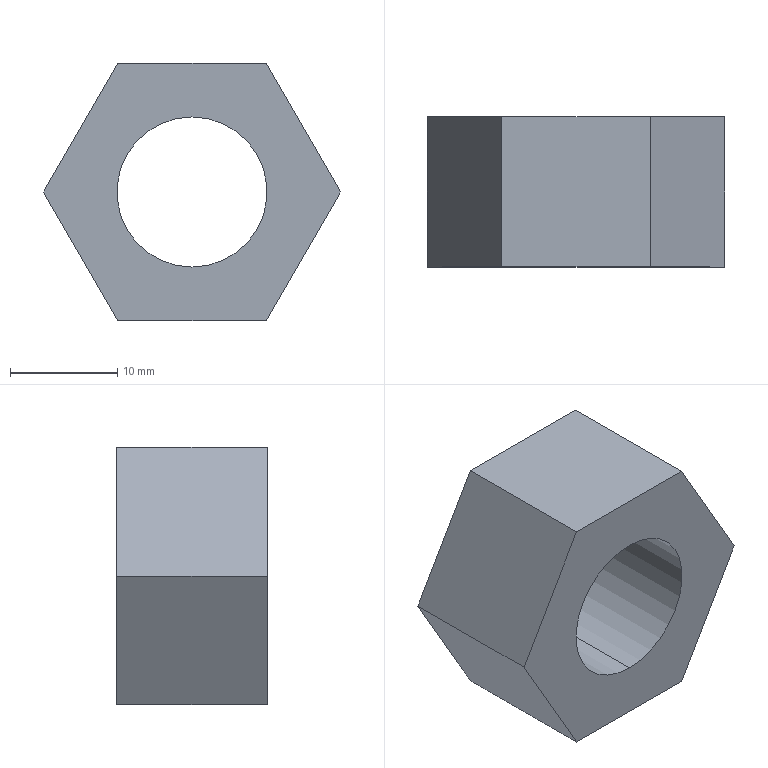Part | STEP file | PN_0077 M16 nut | 1 solid | 10 faces | box 27.713 x 14 x 24 mm | volume 4828 mm3 | plane 8 | cylinder 2 | commonest cylinder face diameters 14 x2
STEP:
#1=CARTESIAN_POINT('',(0.,0.,0.));
#2=DIRECTION('',(0.,0.,1.));
#3=DIRECTION('',(1.,0.,0.));
#4=AXIS2_PLACEMENT_3D('',#1,#2,#3);
#5=CARTESIAN_POINT('',(0.,0.,7.));
#6=VERTEX_POINT('',#5);
#7=CARTESIAN_POINT('',(0.,14.,7.));
#8=VERTEX_POINT('',#7);
#9=CARTESIAN_POINT('',(0.,14.,7.));
#10=DIRECTION('',(0.,1.,0.));
#11=VECTOR('',#10,1.);
#12=LINE('',#9,#11);
#13=CARTESIAN_POINT('',(0.,14.,0.));
#14=DIRECTION('',(0.,1.,0.));
#15=DIRECTION('',(0.,0.,1.));
#16=AXIS2_PLACEMENT_3D('',#13,#14,#15);
#17=CYLINDRICAL_SURFACE('',#16,7.);
#18=CARTESIAN_POINT('',(6.283,0.));
#19=DIRECTION('',(0.,1.));
#20=VECTOR('',#19,1.);
#21=LINE('',#18,#20);
#22=(GEOMETRIC_REPRESENTATION_CONTEXT(2)PARAMETRIC_REPRESENTATION_CONTEXT()REPRESENTATION_CONTEXT('',''));
#23=DEFINITIONAL_REPRESENTATION('',(#21),#22);
#24=PCURVE('',#17,#23);
#25=CARTESIAN_POINT('',(0.,14.,0.));
#26=DIRECTION('',(0.,1.,0.));
#27=DIRECTION('',(0.,0.,1.));
#28=AXIS2_PLACEMENT_3D('',#25,#26,#27);
#29=CYLINDRICAL_SURFACE('',#28,7.);
#30=CARTESIAN_POINT('',(0.,0.));
#31=DIRECTION('',(0.,1.));
#32=VECTOR('',#31,1.);
#33=LINE('',#30,#32);
#34=(GEOMETRIC_REPRESENTATION_CONTEXT(2)PARAMETRIC_REPRESENTATION_CONTEXT()REPRESENTATION_CONTEXT('',''));
#35=DEFINITIONAL_REPRESENTATION('',(#33),#34);
#36=PCURVE('',#29,#35);
#37=SURFACE_CURVE('',#12,(#24,#36),.PCURVE_S1.);
#38=EDGE_CURVE('',#6,#8,#37,.T.);
#39=ORIENTED_EDGE('',*,*,#38,.T.);
#40=CARTESIAN_POINT('',(0.,14.,-7.));
#41=VERTEX_POINT('',#40);
#42=CARTESIAN_POINT('',(0.,14.,0.));
#43=DIRECTION('',(0.,1.,0.));
#44=DIRECTION('',(0.,0.,1.));
#45=AXIS2_PLACEMENT_3D('',#42,#43,#44);
#46=CIRCLE('',#45,7.);
#47=CARTESIAN_POINT('',(0.,0.));
#48=DIRECTION('',(1.,0.));
#49=VECTOR('',#48,1.);
#50=LINE('',#47,#49);
#51=(GEOMETRIC_REPRESENTATION_CONTEXT(2)PARAMETRIC_REPRESENTATION_CONTEXT()REPRESENTATION_CONTEXT('',''));
#52=DEFINITIONAL_REPRESENTATION('',(#50),#51);
#53=PCURVE('',#17,#52);
#54=CARTESIAN_POINT('',(0.,14.,0.));
#55=DIRECTION('',(0.,1.,0.));
#56=DIRECTION('',(0.,0.,1.));
#57=AXIS2_PLACEMENT_3D('',#54,#55,#56);
#58=PLANE('',#57);
#59=CARTESIAN_POINT('',(0.,0.));
#60=DIRECTION('',(1.,0.));
#61=AXIS2_PLACEMENT_2D('',#59,#60);
#62=CIRCLE('',#61,7.);
#63=(GEOMETRIC_REPRESENTATION_CONTEXT(2)PARAMETRIC_REPRESENTATION_CONTEXT()REPRESENTATION_CONTEXT('',''));
#64=DEFINITIONAL_REPRESENTATION('',(#62),#63);
#65=PCURVE('',#58,#64);
#66=SURFACE_CURVE('',#46,(#53,#65),.PCURVE_S1.);
#67=EDGE_CURVE('',#41,#8,#66,.T.);
#68=ORIENTED_EDGE('',*,*,#67,.F.);
#69=CARTESIAN_POINT('',(0.,0.,-7.));
#70=VERTEX_POINT('',#69);
#71=CARTESIAN_POINT('',(0.,14.,-7.));
#72=DIRECTION('',(0.,1.,0.));
#73=VECTOR('',#72,1.);
#74=LINE('',#71,#73);
#75=CARTESIAN_POINT('',(3.142,0.));
#76=DIRECTION('',(0.,1.));
#77=VECTOR('',#76,1.);
#78=LINE('',#75,#77);
#79=(GEOMETRIC_REPRESENTATION_CONTEXT(2)PARAMETRIC_REPRESENTATION_CONTEXT()REPRESENTATION_CONTEXT('',''));
#80=DEFINITIONAL_REPRESENTATION('',(#78),#79);
#81=PCURVE('',#17,#80);
#82=CARTESIAN_POINT('',(3.142,0.));
#83=DIRECTION('',(0.,1.));
#84=VECTOR('',#83,1.);
#85=LINE('',#82,#84);
#86=(GEOMETRIC_REPRESENTATION_CONTEXT(2)PARAMETRIC_REPRESENTATION_CONTEXT()REPRESENTATION_CONTEXT('',''));
#87=DEFINITIONAL_REPRESENTATION('',(#85),#86);
#88=PCURVE('',#29,#87);
#89=SURFACE_CURVE('',#74,(#81,#88),.PCURVE_S1.);
#90=EDGE_CURVE('',#70,#41,#89,.T.);
#91=ORIENTED_EDGE('',*,*,#90,.F.);
#92=CARTESIAN_POINT('',(0.,0.,0.));
#93=DIRECTION('',(0.,1.,0.));
#94=DIRECTION('',(0.,0.,1.));
#95=AXIS2_PLACEMENT_3D('',#92,#93,#94);
#96=CIRCLE('',#95,7.);
#97=CARTESIAN_POINT('',(0.,-14.));
#98=DIRECTION('',(1.,0.));
#99=VECTOR('',#98,1.);
#100=LINE('',#97,#99);
#101=(GEOMETRIC_REPRESENTATION_CONTEXT(2)PARAMETRIC_REPRESENTATION_CONTEXT()REPRESENTATION_CONTEXT('',''));
#102=DEFINITIONAL_REPRESENTATION('',(#100),#101);
#103=PCURVE('',#17,#102);
#104=CARTESIAN_POINT('',(0.,0.,0.));
#105=DIRECTION('',(0.,1.,0.));
#106=DIRECTION('',(0.,0.,1.));
#107=AXIS2_PLACEMENT_3D('',#104,#105,#106);
#108=PLANE('',#107);
#109=CARTESIAN_POINT('',(0.,0.));
#110=DIRECTION('',(1.,0.));
#111=AXIS2_PLACEMENT_2D('',#109,#110);
#112=CIRCLE('',#111,7.);
#113=(GEOMETRIC_REPRESENTATION_CONTEXT(2)PARAMETRIC_REPRESENTATION_CONTEXT()REPRESENTATION_CONTEXT('',''));
#114=DEFINITIONAL_REPRESENTATION('',(#112),#113);
#115=PCURVE('',#108,#114);
#116=SURFACE_CURVE('',#96,(#103,#115),.PCURVE_S1.);
#117=EDGE_CURVE('',#70,#6,#116,.T.);
#118=ORIENTED_EDGE('',*,*,#117,.T.);
#119=EDGE_LOOP('',(#39,#68,#91,#118));
#120=FACE_BOUND('',#119,.F.);
#121=ADVANCED_FACE('',(#120),#17,.F.);
#122=CARTESIAN_POINT('',(6.928,0.,-12.));
#123=VERTEX_POINT('',#122);
#124=CARTESIAN_POINT('',(-6.928,0.,-12.));
#125=VERTEX_POINT('',#124);
#126=CARTESIAN_POINT('',(6.928,0.,-12.));
#127=DIRECTION('',(-1.,0.,0.));
#128=VECTOR('',#127,1.);
#129=LINE('',#126,#128);
#130=CARTESIAN_POINT('',(6.928,14.,-12.));
#131=DIRECTION('',(0.,0.,1.));
#132=DIRECTION('',(1.,0.,0.));
#133=AXIS2_PLACEMENT_3D('',#130,#131,#132);
#134=PLANE('',#133);
#135=CARTESIAN_POINT('',(0.,-14.));
#136=DIRECTION('',(-1.,0.));
#137=VECTOR('',#136,1.);
#138=LINE('',#135,#137);
#139=(GEOMETRIC_REPRESENTATION_CONTEXT(2)PARAMETRIC_REPRESENTATION_CONTEXT()REPRESENTATION_CONTEXT('',''));
#140=DEFINITIONAL_REPRESENTATION('',(#138),#139);
#141=PCURVE('',#134,#140);
#142=CARTESIAN_POINT('',(-12.,6.928));
#143=DIRECTION('',(0.,-1.));
#144=VECTOR('',#143,1.);
#145=LINE('',#142,#144);
#146=(GEOMETRIC_REPRESENTATION_CONTEXT(2)PARAMETRIC_REPRESENTATION_CONTEXT()REPRESENTATION_CONTEXT('',''));
#147=DEFINITIONAL_REPRESENTATION('',(#145),#146);
#148=PCURVE('',#108,#147);
#149=SURFACE_CURVE('',#129,(#141,#148),.PCURVE_S1.);
#150=EDGE_CURVE('',#123,#125,#149,.T.);
#151=ORIENTED_EDGE('',*,*,#150,.T.);
#152=CARTESIAN_POINT('',(-6.928,14.,-12.));
#153=VERTEX_POINT('',#152);
#154=CARTESIAN_POINT('',(-6.928,14.,-12.));
#155=DIRECTION('',(0.,-1.,0.));
#156=VECTOR('',#155,1.);
#157=LINE('',#154,#156);
#158=CARTESIAN_POINT('',(-13.856,0.));
#159=DIRECTION('',(0.,-1.));
#160=VECTOR('',#159,1.);
#161=LINE('',#158,#160);
#162=(GEOMETRIC_REPRESENTATION_CONTEXT(2)PARAMETRIC_REPRESENTATION_CONTEXT()REPRESENTATION_CONTEXT('',''));
#163=DEFINITIONAL_REPRESENTATION('',(#161),#162);
#164=PCURVE('',#134,#163);
#165=CARTESIAN_POINT('',(-6.928,14.,-12.));
#166=DIRECTION('',(0.866,0.,0.5));
#167=DIRECTION('',(0.5,0.,-0.866));
#168=AXIS2_PLACEMENT_3D('',#165,#166,#167);
#169=PLANE('',#168);
#170=CARTESIAN_POINT('',(0.,0.));
#171=DIRECTION('',(0.,-1.));
#172=VECTOR('',#171,1.);
#173=LINE('',#170,#172);
#174=(GEOMETRIC_REPRESENTATION_CONTEXT(2)PARAMETRIC_REPRESENTATION_CONTEXT()REPRESENTATION_CONTEXT('',''));
#175=DEFINITIONAL_REPRESENTATION('',(#173),#174);
#176=PCURVE('',#169,#175);
#177=SURFACE_CURVE('',#157,(#164,#176),.PCURVE_S1.);
#178=EDGE_CURVE('',#153,#125,#177,.T.);
#179=ORIENTED_EDGE('',*,*,#178,.F.);
#180=CARTESIAN_POINT('',(6.928,14.,-12.));
#181=VERTEX_POINT('',#180);
#182=CARTESIAN_POINT('',(6.928,14.,-12.));
#183=DIRECTION('',(-1.,0.,0.));
#184=VECTOR('',#183,1.);
#185=LINE('',#182,#184);
#186=CARTESIAN_POINT('',(0.,0.));
#187=DIRECTION('',(-1.,0.));
#188=VECTOR('',#187,1.);
#189=LINE('',#186,#188);
#190=(GEOMETRIC_REPRESENTATION_CONTEXT(2)PARAMETRIC_REPRESENTATION_CONTEXT()REPRESENTATION_CONTEXT('',''));
#191=DEFINITIONAL_REPRESENTATION('',(#189),#190);
#192=PCURVE('',#134,#191);
#193=CARTESIAN_POINT('',(-12.,6.928));
#194=DIRECTION('',(0.,-1.));
#195=VECTOR('',#194,1.);
#196=LINE('',#193,#195);
#197=(GEOMETRIC_REPRESENTATION_CONTEXT(2)PARAMETRIC_REPRESENTATION_CONTEXT()REPRESENTATION_CONTEXT('',''));
#198=DEFINITIONAL_REPRESENTATION('',(#196),#197);
#199=PCURVE('',#58,#198);
#200=SURFACE_CURVE('',#185,(#192,#199),.PCURVE_S1.);
#201=EDGE_CURVE('',#181,#153,#200,.T.);
#202=ORIENTED_EDGE('',*,*,#201,.F.);
#203=CARTESIAN_POINT('',(6.928,14.,-12.));
#204=DIRECTION('',(0.,-1.,0.));
#205=VECTOR('',#204,1.);
#206=LINE('',#203,#205);
#207=CARTESIAN_POINT('',(0.,0.));
#208=DIRECTION('',(0.,-1.));
#209=VECTOR('',#208,1.);
#210=LINE('',#207,#209);
#211=(GEOMETRIC_REPRESENTATION_CONTEXT(2)PARAMETRIC_REPRESENTATION_CONTEXT()REPRESENTATION_CONTEXT('',''));
#212=DEFINITIONAL_REPRESENTATION('',(#210),#211);
#213=PCURVE('',#134,#212);
#214=CARTESIAN_POINT('',(13.856,14.,0.));
#215=DIRECTION('',(-0.866,0.,0.5));
#216=DIRECTION('',(0.5,0.,0.866));
#217=AXIS2_PLACEMENT_3D('',#214,#215,#216);
#218=PLANE('',#217);
#219=CARTESIAN_POINT('',(-13.856,0.));
#220=DIRECTION('',(0.,-1.));
#221=VECTOR('',#220,1.);
#222=LINE('',#219,#221);
#223=(GEOMETRIC_REPRESENTATION_CONTEXT(2)PARAMETRIC_REPRESENTATION_CONTEXT()REPRESENTATION_CONTEXT('',''));
#224=DEFINITIONAL_REPRESENTATION('',(#222),#223);
#225=PCURVE('',#218,#224);
#226=SURFACE_CURVE('',#206,(#213,#225),.PCURVE_S1.);
#227=EDGE_CURVE('',#181,#123,#226,.T.);
#228=ORIENTED_EDGE('',*,*,#227,.T.);
#229=EDGE_LOOP('',(#151,#179,#202,#228));
#230=FACE_BOUND('',#229,.T.);
#231=ADVANCED_FACE('',(#230),#134,.F.);
#232=CARTESIAN_POINT('',(-13.856,0.,0.));
#233=VERTEX_POINT('',#232);
#234=CARTESIAN_POINT('',(-6.928,0.,-12.));
#235=DIRECTION('',(-0.5,0.,0.866));
#236=VECTOR('',#235,1.);
#237=LINE('',#234,#236);
#238=CARTESIAN_POINT('',(0.,-14.));
#239=DIRECTION('',(-1.,0.));
#240=VECTOR('',#239,1.);
#241=LINE('',#238,#240);
#242=(GEOMETRIC_REPRESENTATION_CONTEXT(2)PARAMETRIC_REPRESENTATION_CONTEXT()REPRESENTATION_CONTEXT('',''));
#243=DEFINITIONAL_REPRESENTATION('',(#241),#242);
#244=PCURVE('',#169,#243);
#245=CARTESIAN_POINT('',(-12.,-6.928));
#246=DIRECTION('',(0.866,-0.5));
#247=VECTOR('',#246,1.);
#248=LINE('',#245,#247);
#249=(GEOMETRIC_REPRESENTATION_CONTEXT(2)PARAMETRIC_REPRESENTATION_CONTEXT()REPRESENTATION_CONTEXT('',''));
#250=DEFINITIONAL_REPRESENTATION('',(#248),#249);
#251=PCURVE('',#108,#250);
#252=SURFACE_CURVE('',#237,(#244,#251),.PCURVE_S1.);
#253=EDGE_CURVE('',#125,#233,#252,.T.);
#254=ORIENTED_EDGE('',*,*,#253,.T.);
#255=CARTESIAN_POINT('',(-13.856,14.,0.));
#256=VERTEX_POINT('',#255);
#257=CARTESIAN_POINT('',(-13.856,14.,0.));
#258=DIRECTION('',(0.,-1.,0.));
#259=VECTOR('',#258,1.);
#260=LINE('',#257,#259);
#261=CARTESIAN_POINT('',(-13.856,0.));
#262=DIRECTION('',(0.,-1.));
#263=VECTOR('',#262,1.);
#264=LINE('',#261,#263);
#265=(GEOMETRIC_REPRESENTATION_CONTEXT(2)PARAMETRIC_REPRESENTATION_CONTEXT()REPRESENTATION_CONTEXT('',''));
#266=DEFINITIONAL_REPRESENTATION('',(#264),#265);
#267=PCURVE('',#169,#266);
#268=CARTESIAN_POINT('',(-13.856,14.,0.));
#269=DIRECTION('',(0.866,0.,-0.5));
#270=DIRECTION('',(-0.5,0.,-0.866));
#271=AXIS2_PLACEMENT_3D('',#268,#269,#270);
#272=PLANE('',#271);
#273=CARTESIAN_POINT('',(0.,0.));
#274=DIRECTION('',(0.,-1.));
#275=VECTOR('',#274,1.);
#276=LINE('',#273,#275);
#277=(GEOMETRIC_REPRESENTATION_CONTEXT(2)PARAMETRIC_REPRESENTATION_CONTEXT()REPRESENTATION_CONTEXT('',''));
#278=DEFINITIONAL_REPRESENTATION('',(#276),#277);
#279=PCURVE('',#272,#278);
#280=SURFACE_CURVE('',#260,(#267,#279),.PCURVE_S1.);
#281=EDGE_CURVE('',#256,#233,#280,.T.);
#282=ORIENTED_EDGE('',*,*,#281,.F.);
#283=CARTESIAN_POINT('',(-6.928,14.,-12.));
#284=DIRECTION('',(-0.5,0.,0.866));
#285=VECTOR('',#284,1.);
#286=LINE('',#283,#285);
#287=CARTESIAN_POINT('',(0.,0.));
#288=DIRECTION('',(-1.,0.));
#289=VECTOR('',#288,1.);
#290=LINE('',#287,#289);
#291=(GEOMETRIC_REPRESENTATION_CONTEXT(2)PARAMETRIC_REPRESENTATION_CONTEXT()REPRESENTATION_CONTEXT('',''));
#292=DEFINITIONAL_REPRESENTATION('',(#290),#291);
#293=PCURVE('',#169,#292);
#294=CARTESIAN_POINT('',(-12.,-6.928));
#295=DIRECTION('',(0.866,-0.5));
#296=VECTOR('',#295,1.);
#297=LINE('',#294,#296);
#298=(GEOMETRIC_REPRESENTATION_CONTEXT(2)PARAMETRIC_REPRESENTATION_CONTEXT()REPRESENTATION_CONTEXT('',''));
#299=DEFINITIONAL_REPRESENTATION('',(#297),#298);
#300=PCURVE('',#58,#299);
#301=SURFACE_CURVE('',#286,(#293,#300),.PCURVE_S1.);
#302=EDGE_CURVE('',#153,#256,#301,.T.);
#303=ORIENTED_EDGE('',*,*,#302,.F.);
#304=ORIENTED_EDGE('',*,*,#178,.T.);
#305=EDGE_LOOP('',(#254,#282,#303,#304));
#306=FACE_BOUND('',#305,.T.);
#307=ADVANCED_FACE('',(#306),#169,.F.);
#308=CARTESIAN_POINT('',(-6.928,0.,12.));
#309=VERTEX_POINT('',#308);
#310=CARTESIAN_POINT('',(-13.856,0.,0.));
#311=DIRECTION('',(0.5,0.,0.866));
#312=VECTOR('',#311,1.);
#313=LINE('',#310,#312);
#314=CARTESIAN_POINT('',(0.,-14.));
#315=DIRECTION('',(-1.,0.));
#316=VECTOR('',#315,1.);
#317=LINE('',#314,#316);
#318=(GEOMETRIC_REPRESENTATION_CONTEXT(2)PARAMETRIC_REPRESENTATION_CONTEXT()REPRESENTATION_CONTEXT('',''));
#319=DEFINITIONAL_REPRESENTATION('',(#317),#318);
#320=PCURVE('',#272,#319);
#321=CARTESIAN_POINT('',(0.,-13.856));
#322=DIRECTION('',(0.866,0.5));
#323=VECTOR('',#322,1.);
#324=LINE('',#321,#323);
#325=(GEOMETRIC_REPRESENTATION_CONTEXT(2)PARAMETRIC_REPRESENTATION_CONTEXT()REPRESENTATION_CONTEXT('',''));
#326=DEFINITIONAL_REPRESENTATION('',(#324),#325);
#327=PCURVE('',#108,#326);
#328=SURFACE_CURVE('',#313,(#320,#327),.PCURVE_S1.);
#329=EDGE_CURVE('',#233,#309,#328,.T.);
#330=ORIENTED_EDGE('',*,*,#329,.T.);
#331=CARTESIAN_POINT('',(-6.928,14.,12.));
#332=VERTEX_POINT('',#331);
#333=CARTESIAN_POINT('',(-6.928,14.,12.));
#334=DIRECTION('',(0.,-1.,0.));
#335=VECTOR('',#334,1.);
#336=LINE('',#333,#335);
#337=CARTESIAN_POINT('',(-13.856,0.));
#338=DIRECTION('',(0.,-1.));
#339=VECTOR('',#338,1.);
#340=LINE('',#337,#339);
#341=(GEOMETRIC_REPRESENTATION_CONTEXT(2)PARAMETRIC_REPRESENTATION_CONTEXT()REPRESENTATION_CONTEXT('',''));
#342=DEFINITIONAL_REPRESENTATION('',(#340),#341);
#343=PCURVE('',#272,#342);
#344=CARTESIAN_POINT('',(-6.928,14.,12.));
#345=DIRECTION('',(0.,0.,-1.));
#346=DIRECTION('',(-1.,0.,0.));
#347=AXIS2_PLACEMENT_3D('',#344,#345,#346);
#348=PLANE('',#347);
#349=CARTESIAN_POINT('',(0.,0.));
#350=DIRECTION('',(0.,-1.));
#351=VECTOR('',#350,1.);
#352=LINE('',#349,#351);
#353=(GEOMETRIC_REPRESENTATION_CONTEXT(2)PARAMETRIC_REPRESENTATION_CONTEXT()REPRESENTATION_CONTEXT('',''));
#354=DEFINITIONAL_REPRESENTATION('',(#352),#353);
#355=PCURVE('',#348,#354);
#356=SURFACE_CURVE('',#336,(#343,#355),.PCURVE_S1.);
#357=EDGE_CURVE('',#332,#309,#356,.T.);
#358=ORIENTED_EDGE('',*,*,#357,.F.);
#359=CARTESIAN_POINT('',(-13.856,14.,0.));
#360=DIRECTION('',(0.5,0.,0.866));
#361=VECTOR('',#360,1.);
#362=LINE('',#359,#361);
#363=CARTESIAN_POINT('',(0.,0.));
#364=DIRECTION('',(-1.,0.));
#365=VECTOR('',#364,1.);
#366=LINE('',#363,#365);
#367=(GEOMETRIC_REPRESENTATION_CONTEXT(2)PARAMETRIC_REPRESENTATION_CONTEXT()REPRESENTATION_CONTEXT('',''));
#368=DEFINITIONAL_REPRESENTATION('',(#366),#367);
#369=PCURVE('',#272,#368);
#370=CARTESIAN_POINT('',(0.,-13.856));
#371=DIRECTION('',(0.866,0.5));
#372=VECTOR('',#371,1.);
#373=LINE('',#370,#372);
#374=(GEOMETRIC_REPRESENTATION_CONTEXT(2)PARAMETRIC_REPRESENTATION_CONTEXT()REPRESENTATION_CONTEXT('',''));
#375=DEFINITIONAL_REPRESENTATION('',(#373),#374);
#376=PCURVE('',#58,#375);
#377=SURFACE_CURVE('',#362,(#369,#376),.PCURVE_S1.);
#378=EDGE_CURVE('',#256,#332,#377,.T.);
#379=ORIENTED_EDGE('',*,*,#378,.F.);
#380=ORIENTED_EDGE('',*,*,#281,.T.);
#381=EDGE_LOOP('',(#330,#358,#379,#380));
#382=FACE_BOUND('',#381,.T.);
#383=ADVANCED_FACE('',(#382),#272,.F.);
#384=CARTESIAN_POINT('',(6.928,0.,12.));
#385=VERTEX_POINT('',#384);
#386=CARTESIAN_POINT('',(-6.928,0.,12.));
#387=DIRECTION('',(1.,0.,0.));
#388=VECTOR('',#387,1.);
#389=LINE('',#386,#388);
#390=CARTESIAN_POINT('',(0.,-14.));
#391=DIRECTION('',(-1.,0.));
#392=VECTOR('',#391,1.);
#393=LINE('',#390,#392);
#394=(GEOMETRIC_REPRESENTATION_CONTEXT(2)PARAMETRIC_REPRESENTATION_CONTEXT()REPRESENTATION_CONTEXT('',''));
#395=DEFINITIONAL_REPRESENTATION('',(#393),#394);
#396=PCURVE('',#348,#395);
#397=CARTESIAN_POINT('',(12.,-6.928));
#398=DIRECTION('',(0.,1.));
#399=VECTOR('',#398,1.);
#400=LINE('',#397,#399);
#401=(GEOMETRIC_REPRESENTATION_CONTEXT(2)PARAMETRIC_REPRESENTATION_CONTEXT()REPRESENTATION_CONTEXT('',''));
#402=DEFINITIONAL_REPRESENTATION('',(#400),#401);
#403=PCURVE('',#108,#402);
#404=SURFACE_CURVE('',#389,(#396,#403),.PCURVE_S1.);
#405=EDGE_CURVE('',#309,#385,#404,.T.);
#406=ORIENTED_EDGE('',*,*,#405,.T.);
#407=CARTESIAN_POINT('',(6.928,14.,12.));
#408=VERTEX_POINT('',#407);
#409=CARTESIAN_POINT('',(6.928,14.,12.));
#410=DIRECTION('',(0.,-1.,0.));
#411=VECTOR('',#410,1.);
#412=LINE('',#409,#411);
#413=CARTESIAN_POINT('',(-13.856,0.));
#414=DIRECTION('',(0.,-1.));
#415=VECTOR('',#414,1.);
#416=LINE('',#413,#415);
#417=(GEOMETRIC_REPRESENTATION_CONTEXT(2)PARAMETRIC_REPRESENTATION_CONTEXT()REPRESENTATION_CONTEXT('',''));
#418=DEFINITIONAL_REPRESENTATION('',(#416),#417);
#419=PCURVE('',#348,#418);
#420=CARTESIAN_POINT('',(6.928,14.,12.));
#421=DIRECTION('',(-0.866,0.,-0.5));
#422=DIRECTION('',(-0.5,0.,0.866));
#423=AXIS2_PLACEMENT_3D('',#420,#421,#422);
#424=PLANE('',#423);
#425=CARTESIAN_POINT('',(0.,0.));
#426=DIRECTION('',(0.,-1.));
#427=VECTOR('',#426,1.);
#428=LINE('',#425,#427);
#429=(GEOMETRIC_REPRESENTATION_CONTEXT(2)PARAMETRIC_REPRESENTATION_CONTEXT()REPRESENTATION_CONTEXT('',''));
#430=DEFINITIONAL_REPRESENTATION('',(#428),#429);
#431=PCURVE('',#424,#430);
#432=SURFACE_CURVE('',#412,(#419,#431),.PCURVE_S1.);
#433=EDGE_CURVE('',#408,#385,#432,.T.);
#434=ORIENTED_EDGE('',*,*,#433,.F.);
#435=CARTESIAN_POINT('',(-6.928,14.,12.));
#436=DIRECTION('',(1.,0.,0.));
#437=VECTOR('',#436,1.);
#438=LINE('',#435,#437);
#439=CARTESIAN_POINT('',(0.,0.));
#440=DIRECTION('',(-1.,0.));
#441=VECTOR('',#440,1.);
#442=LINE('',#439,#441);
#443=(GEOMETRIC_REPRESENTATION_CONTEXT(2)PARAMETRIC_REPRESENTATION_CONTEXT()REPRESENTATION_CONTEXT('',''));
#444=DEFINITIONAL_REPRESENTATION('',(#442),#443);
#445=PCURVE('',#348,#444);
#446=CARTESIAN_POINT('',(12.,-6.928));
#447=DIRECTION('',(0.,1.));
#448=VECTOR('',#447,1.);
#449=LINE('',#446,#448);
#450=(GEOMETRIC_REPRESENTATION_CONTEXT(2)PARAMETRIC_REPRESENTATION_CONTEXT()REPRESENTATION_CONTEXT('',''));
#451=DEFINITIONAL_REPRESENTATION('',(#449),#450);
#452=PCURVE('',#58,#451);
#453=SURFACE_CURVE('',#438,(#445,#452),.PCURVE_S1.);
#454=EDGE_CURVE('',#332,#408,#453,.T.);
#455=ORIENTED_EDGE('',*,*,#454,.F.);
#456=ORIENTED_EDGE('',*,*,#357,.T.);
#457=EDGE_LOOP('',(#406,#434,#455,#456));
#458=FACE_BOUND('',#457,.T.);
#459=ADVANCED_FACE('',(#458),#348,.F.);
#460=CARTESIAN_POINT('',(13.856,0.,0.));
#461=VERTEX_POINT('',#460);
#462=CARTESIAN_POINT('',(6.928,0.,12.));
#463=DIRECTION('',(0.5,0.,-0.866));
#464=VECTOR('',#463,1.);
#465=LINE('',#462,#464);
#466=CARTESIAN_POINT('',(0.,-14.));
#467=DIRECTION('',(-1.,0.));
#468=VECTOR('',#467,1.);
#469=LINE('',#466,#468);
#470=(GEOMETRIC_REPRESENTATION_CONTEXT(2)PARAMETRIC_REPRESENTATION_CONTEXT()REPRESENTATION_CONTEXT('',''));
#471=DEFINITIONAL_REPRESENTATION('',(#469),#470);
#472=PCURVE('',#424,#471);
#473=CARTESIAN_POINT('',(12.,6.928));
#474=DIRECTION('',(-0.866,0.5));
#475=VECTOR('',#474,1.);
#476=LINE('',#473,#475);
#477=(GEOMETRIC_REPRESENTATION_CONTEXT(2)PARAMETRIC_REPRESENTATION_CONTEXT()REPRESENTATION_CONTEXT('',''));
#478=DEFINITIONAL_REPRESENTATION('',(#476),#477);
#479=PCURVE('',#108,#478);
#480=SURFACE_CURVE('',#465,(#472,#479),.PCURVE_S1.);
#481=EDGE_CURVE('',#385,#461,#480,.T.);
#482=ORIENTED_EDGE('',*,*,#481,.T.);
#483=CARTESIAN_POINT('',(13.856,14.,0.));
#484=VERTEX_POINT('',#483);
#485=CARTESIAN_POINT('',(13.856,14.,0.));
#486=DIRECTION('',(0.,-1.,0.));
#487=VECTOR('',#486,1.);
#488=LINE('',#485,#487);
#489=CARTESIAN_POINT('',(-13.856,0.));
#490=DIRECTION('',(0.,-1.));
#491=VECTOR('',#490,1.);
#492=LINE('',#489,#491);
#493=(GEOMETRIC_REPRESENTATION_CONTEXT(2)PARAMETRIC_REPRESENTATION_CONTEXT()REPRESENTATION_CONTEXT('',''));
#494=DEFINITIONAL_REPRESENTATION('',(#492),#493);
#495=PCURVE('',#424,#494);
#496=CARTESIAN_POINT('',(0.,0.));
#497=DIRECTION('',(0.,-1.));
#498=VECTOR('',#497,1.);
#499=LINE('',#496,#498);
#500=(GEOMETRIC_REPRESENTATION_CONTEXT(2)PARAMETRIC_REPRESENTATION_CONTEXT()REPRESENTATION_CONTEXT('',''));
#501=DEFINITIONAL_REPRESENTATION('',(#499),#500);
#502=PCURVE('',#218,#501);
#503=SURFACE_CURVE('',#488,(#495,#502),.PCURVE_S1.);
#504=EDGE_CURVE('',#484,#461,#503,.T.);
#505=ORIENTED_EDGE('',*,*,#504,.F.);
#506=CARTESIAN_POINT('',(6.928,14.,12.));
#507=DIRECTION('',(0.5,0.,-0.866));
#508=VECTOR('',#507,1.);
#509=LINE('',#506,#508);
#510=CARTESIAN_POINT('',(0.,0.));
#511=DIRECTION('',(-1.,0.));
#512=VECTOR('',#511,1.);
#513=LINE('',#510,#512);
#514=(GEOMETRIC_REPRESENTATION_CONTEXT(2)PARAMETRIC_REPRESENTATION_CONTEXT()REPRESENTATION_CONTEXT('',''));
#515=DEFINITIONAL_REPRESENTATION('',(#513),#514);
#516=PCURVE('',#424,#515);
#517=CARTESIAN_POINT('',(12.,6.928));
#518=DIRECTION('',(-0.866,0.5));
#519=VECTOR('',#518,1.);
#520=LINE('',#517,#519);
#521=(GEOMETRIC_REPRESENTATION_CONTEXT(2)PARAMETRIC_REPRESENTATION_CONTEXT()REPRESENTATION_CONTEXT('',''));
#522=DEFINITIONAL_REPRESENTATION('',(#520),#521);
#523=PCURVE('',#58,#522);
#524=SURFACE_CURVE('',#509,(#516,#523),.PCURVE_S1.);
#525=EDGE_CURVE('',#408,#484,#524,.T.);
#526=ORIENTED_EDGE('',*,*,#525,.F.);
#527=ORIENTED_EDGE('',*,*,#433,.T.);
#528=EDGE_LOOP('',(#482,#505,#526,#527));
#529=FACE_BOUND('',#528,.T.);
#530=ADVANCED_FACE('',(#529),#424,.F.);
#531=CARTESIAN_POINT('',(13.856,0.,0.));
#532=DIRECTION('',(-0.5,0.,-0.866));
#533=VECTOR('',#532,1.);
#534=LINE('',#531,#533);
#535=CARTESIAN_POINT('',(0.,-14.));
#536=DIRECTION('',(-1.,0.));
#537=VECTOR('',#536,1.);
#538=LINE('',#535,#537);
#539=(GEOMETRIC_REPRESENTATION_CONTEXT(2)PARAMETRIC_REPRESENTATION_CONTEXT()REPRESENTATION_CONTEXT('',''));
#540=DEFINITIONAL_REPRESENTATION('',(#538),#539);
#541=PCURVE('',#218,#540);
#542=CARTESIAN_POINT('',(0.,13.856));
#543=DIRECTION('',(-0.866,-0.5));
#544=VECTOR('',#543,1.);
#545=LINE('',#542,#544);
#546=(GEOMETRIC_REPRESENTATION_CONTEXT(2)PARAMETRIC_REPRESENTATION_CONTEXT()REPRESENTATION_CONTEXT('',''));
#547=DEFINITIONAL_REPRESENTATION('',(#545),#546);
#548=PCURVE('',#108,#547);
#549=SURFACE_CURVE('',#534,(#541,#548),.PCURVE_S1.);
#550=EDGE_CURVE('',#461,#123,#549,.T.);
#551=ORIENTED_EDGE('',*,*,#550,.T.);
#552=ORIENTED_EDGE('',*,*,#227,.F.);
#553=CARTESIAN_POINT('',(13.856,14.,0.));
#554=DIRECTION('',(-0.5,0.,-0.866));
#555=VECTOR('',#554,1.);
#556=LINE('',#553,#555);
#557=CARTESIAN_POINT('',(0.,0.));
#558=DIRECTION('',(-1.,0.));
#559=VECTOR('',#558,1.);
#560=LINE('',#557,#559);
#561=(GEOMETRIC_REPRESENTATION_CONTEXT(2)PARAMETRIC_REPRESENTATION_CONTEXT()REPRESENTATION_CONTEXT('',''));
#562=DEFINITIONAL_REPRESENTATION('',(#560),#561);
#563=PCURVE('',#218,#562);
#564=CARTESIAN_POINT('',(0.,13.856));
#565=DIRECTION('',(-0.866,-0.5));
#566=VECTOR('',#565,1.);
#567=LINE('',#564,#566);
#568=(GEOMETRIC_REPRESENTATION_CONTEXT(2)PARAMETRIC_REPRESENTATION_CONTEXT()REPRESENTATION_CONTEXT('',''));
#569=DEFINITIONAL_REPRESENTATION('',(#567),#568);
#570=PCURVE('',#58,#569);
#571=SURFACE_CURVE('',#556,(#563,#570),.PCURVE_S1.);
#572=EDGE_CURVE('',#484,#181,#571,.T.);
#573=ORIENTED_EDGE('',*,*,#572,.F.);
#574=ORIENTED_EDGE('',*,*,#504,.T.);
#575=EDGE_LOOP('',(#551,#552,#573,#574));
#576=FACE_BOUND('',#575,.T.);
#577=ADVANCED_FACE('',(#576),#218,.F.);
#578=CARTESIAN_POINT('',(0.,14.,0.));
#579=DIRECTION('',(0.,1.,0.));
#580=DIRECTION('',(0.,0.,1.));
#581=AXIS2_PLACEMENT_3D('',#578,#579,#580);
#582=CIRCLE('',#581,7.);
#583=CARTESIAN_POINT('',(0.,0.));
#584=DIRECTION('',(1.,0.));
#585=AXIS2_PLACEMENT_2D('',#583,#584);
#586=CIRCLE('',#585,7.);
#587=(GEOMETRIC_REPRESENTATION_CONTEXT(2)PARAMETRIC_REPRESENTATION_CONTEXT()REPRESENTATION_CONTEXT('',''));
#588=DEFINITIONAL_REPRESENTATION('',(#586),#587);
#589=PCURVE('',#58,#588);
#590=CARTESIAN_POINT('',(0.,0.));
#591=DIRECTION('',(1.,0.));
#592=VECTOR('',#591,1.);
#593=LINE('',#590,#592);
#594=(GEOMETRIC_REPRESENTATION_CONTEXT(2)PARAMETRIC_REPRESENTATION_CONTEXT()REPRESENTATION_CONTEXT('',''));
#595=DEFINITIONAL_REPRESENTATION('',(#593),#594);
#596=PCURVE('',#29,#595);
#597=SURFACE_CURVE('',#582,(#589,#596),.PCURVE_S1.);
#598=EDGE_CURVE('',#8,#41,#597,.T.);
#599=ORIENTED_EDGE('',*,*,#598,.F.);
#600=ORIENTED_EDGE('',*,*,#67,.F.);
#601=EDGE_LOOP('',(#599,#600));
#602=FACE_BOUND('',#601,.T.);
#603=ORIENTED_EDGE('',*,*,#201,.T.);
#604=ORIENTED_EDGE('',*,*,#302,.T.);
#605=ORIENTED_EDGE('',*,*,#378,.T.);
#606=ORIENTED_EDGE('',*,*,#454,.T.);
#607=ORIENTED_EDGE('',*,*,#525,.T.);
#608=ORIENTED_EDGE('',*,*,#572,.T.);
#609=EDGE_LOOP('',(#603,#604,#605,#606,#607,#608));
#610=FACE_BOUND('',#609,.T.);
#611=ADVANCED_FACE('',(#602,#610),#58,.T.);
#612=CARTESIAN_POINT('',(0.,0.,0.));
#613=DIRECTION('',(0.,1.,0.));
#614=DIRECTION('',(0.,0.,1.));
#615=AXIS2_PLACEMENT_3D('',#612,#613,#614);
#616=CIRCLE('',#615,7.);
#617=CARTESIAN_POINT('',(0.,0.));
#618=DIRECTION('',(1.,0.));
#619=AXIS2_PLACEMENT_2D('',#617,#618);
#620=CIRCLE('',#619,7.);
#621=(GEOMETRIC_REPRESENTATION_CONTEXT(2)PARAMETRIC_REPRESENTATION_CONTEXT()REPRESENTATION_CONTEXT('',''));
#622=DEFINITIONAL_REPRESENTATION('',(#620),#621);
#623=PCURVE('',#108,#622);
#624=CARTESIAN_POINT('',(0.,-14.));
#625=DIRECTION('',(1.,0.));
#626=VECTOR('',#625,1.);
#627=LINE('',#624,#626);
#628=(GEOMETRIC_REPRESENTATION_CONTEXT(2)PARAMETRIC_REPRESENTATION_CONTEXT()REPRESENTATION_CONTEXT('',''));
#629=DEFINITIONAL_REPRESENTATION('',(#627),#628);
#630=PCURVE('',#29,#629);
#631=SURFACE_CURVE('',#616,(#623,#630),.PCURVE_S1.);
#632=EDGE_CURVE('',#6,#70,#631,.T.);
#633=ORIENTED_EDGE('',*,*,#632,.T.);
#634=ORIENTED_EDGE('',*,*,#117,.T.);
#635=EDGE_LOOP('',(#633,#634));
#636=FACE_BOUND('',#635,.T.);
#637=ORIENTED_EDGE('',*,*,#150,.F.);
#638=ORIENTED_EDGE('',*,*,#550,.F.);
#639=ORIENTED_EDGE('',*,*,#481,.F.);
#640=ORIENTED_EDGE('',*,*,#405,.F.);
#641=ORIENTED_EDGE('',*,*,#329,.F.);
#642=ORIENTED_EDGE('',*,*,#253,.F.);
#643=EDGE_LOOP('',(#637,#638,#639,#640,#641,#642));
#644=FACE_BOUND('',#643,.T.);
#645=ADVANCED_FACE('',(#636,#644),#108,.F.);
#646=ORIENTED_EDGE('',*,*,#598,.F.);
#647=ORIENTED_EDGE('',*,*,#38,.F.);
#648=ORIENTED_EDGE('',*,*,#632,.T.);
#649=ORIENTED_EDGE('',*,*,#90,.T.);
#650=EDGE_LOOP('',(#646,#647,#648,#649));
#651=FACE_BOUND('',#650,.F.);
#652=ADVANCED_FACE('',(#651),#29,.F.);
#653=CLOSED_SHELL('',(#121,#231,#307,#383,#459,#530,#577,#611,#645,#652));
#654=MANIFOLD_SOLID_BREP('',#653);
#655=(LENGTH_UNIT()NAMED_UNIT(*)SI_UNIT(.MILLI.,.METRE.));
#656=UNCERTAINTY_MEASURE_WITH_UNIT(LENGTH_MEASURE(0.0000001),#655,'','');
#657=(NAMED_UNIT(*)PLANE_ANGLE_UNIT()SI_UNIT($,.RADIAN.));
#658=(NAMED_UNIT(*)SI_UNIT($,.STERADIAN.)SOLID_ANGLE_UNIT());
#659=(GEOMETRIC_REPRESENTATION_CONTEXT(3)GLOBAL_UNCERTAINTY_ASSIGNED_CONTEXT((#656))GLOBAL_UNIT_ASSIGNED_CONTEXT((#655,#657,#658))REPRESENTATION_CONTEXT('',''));
#660=ADVANCED_BREP_SHAPE_REPRESENTATION('',(#4,#654),#659);